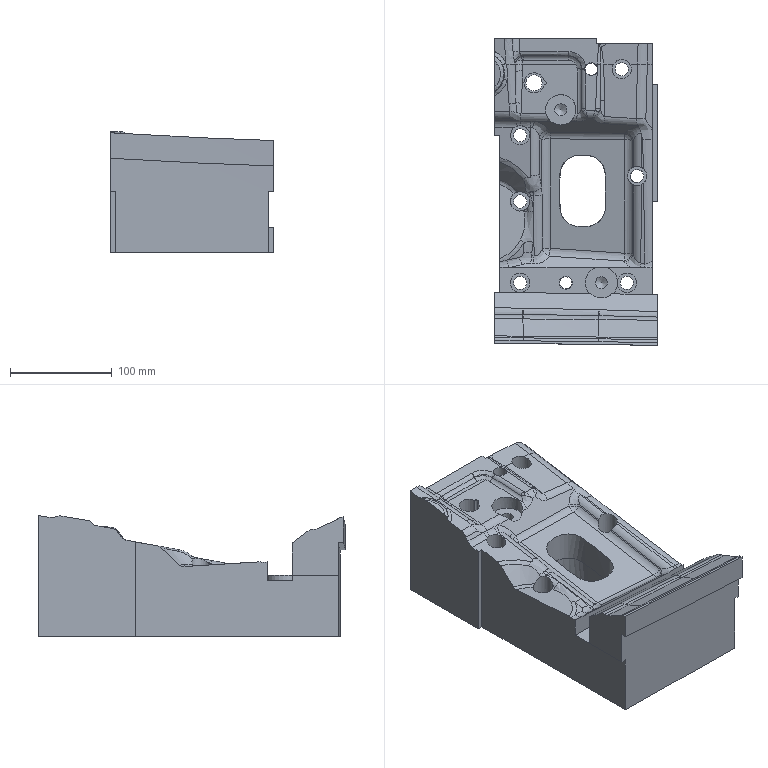Part | NX | features solid 2 | 1 solid | 219 faces | box 160.001 x 301.636 x 118.894 mm | volume 3423228 mm3 | spline 82 | cylinder 75 | plane 56 | sphere 4 | cone 2 | commonest cylinder face diameters 20 x28 13 x8 10 x6 19 x6 30 x5 12 x4